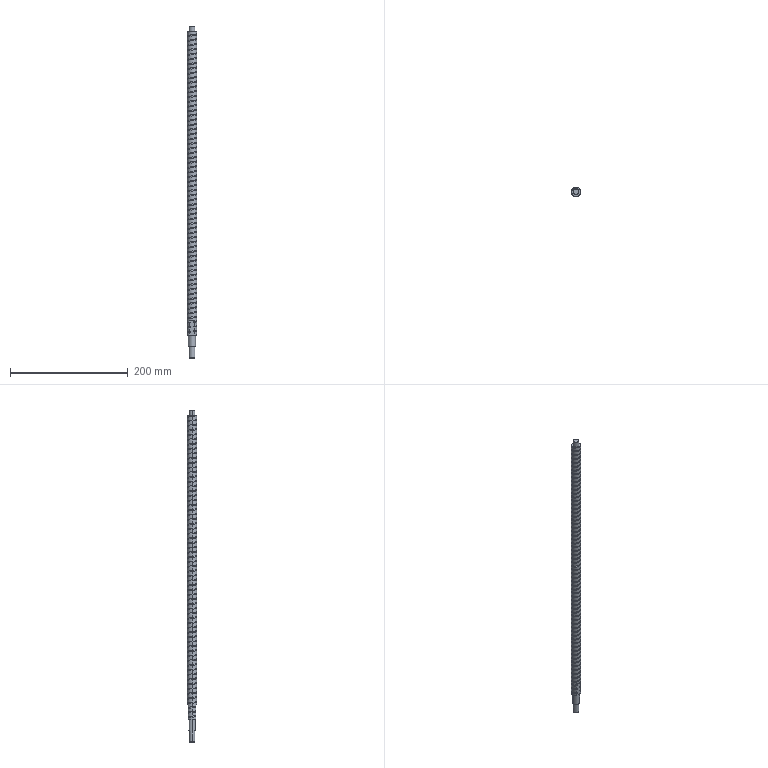Part | STEP file | 1 solid | 168 faces | box 16 x 16 x 565 mm | volume 102973 mm3 | cylinder 145 | plane 12 | spline 7 | cone 4 | commonest cylinder face diameters 16 x135 3 x4 10 x4 12 x2